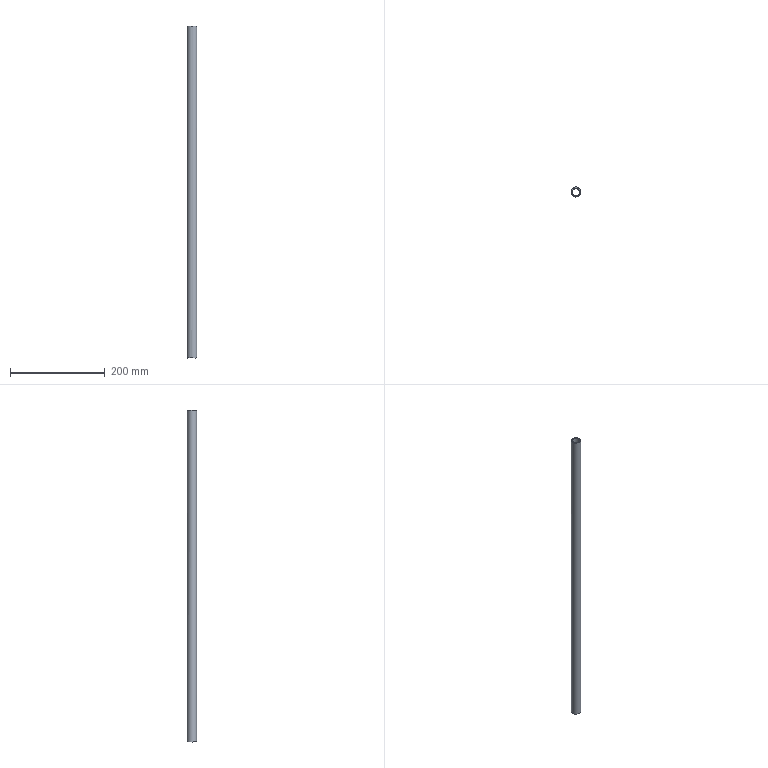Part | STEP file | 1 solid | 4 faces | box 20 x 20 x 700 mm | volume 96209 mm3 | cylinder 3 | plane 1 | commonest cylinder face diameters 15 x1 20 x1 700 x1